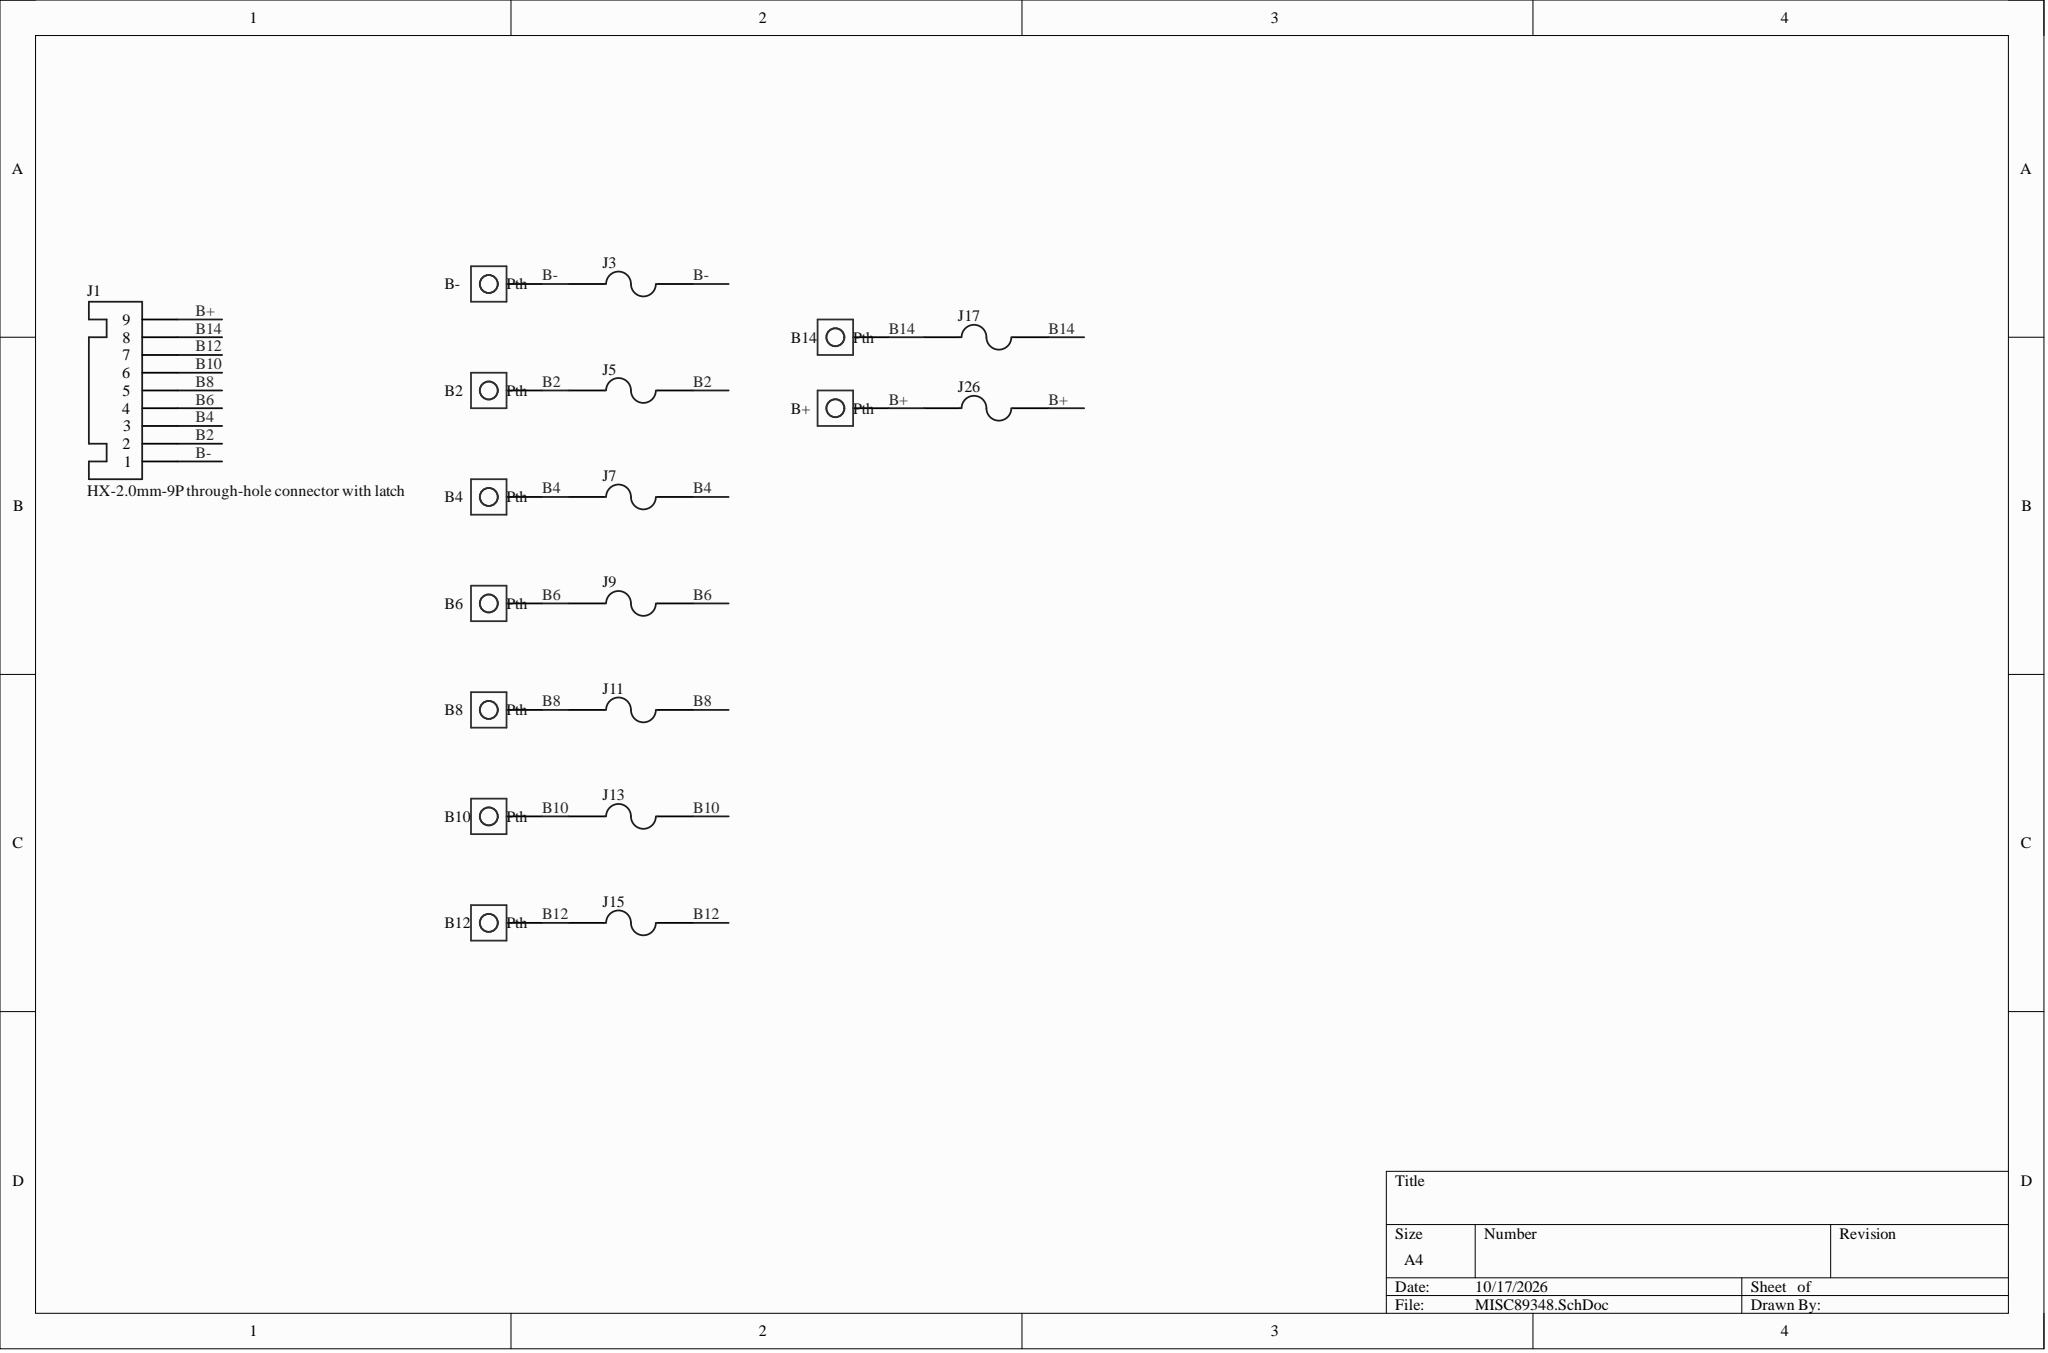Circuit board | Altium Designer | 19 parts | 9 nets
Bill of materials:
Comment,Description,Designator,Footprint,LibRef,Quantity
"Pth","Through-hole pad","B2, B4, B6, B10, B12, B14, B-, B+","55*10*1MM","Pth","8"
"Pth","Through-hole pad","B8","161.5*10*1MM","Pth","1"
"HX-2.0mm-9P through-hole connector with latch","HX-2.54mm-9P through-hole connector with latch","J1","HX2.0-9P","HX-2.54mm-9P直插带扣","1"
"FPC","","J3, J5, J7, J9, J11, J13, J15, J17, J26","异形电阻","FPC","9"
Netlist (Protel format):
[
B2
55*10*1MM
Pth



]
[
B4
55*10*1MM
Pth



]
[
B6
55*10*1MM
Pth



]
[
B8
161.5*10*1MM
Pth



]
[
B10
55*10*1MM
Pth



]
[
B12
55*10*1MM
Pth



]
[
B14
55*10*1MM
Pth



]
[
B+
55*10*1MM
Pth



]
[
B-
55*10*1MM
Pth



]
[
J1
HX2.0-9P
HX-2.0mm-9P through-hole connector with latch



]
[
J3
异形电阻
FPC



]
[
J5
异形电阻
FPC



]
[
J7
异形电阻
FPC



]
[
J9
异形电阻
FPC



]
[
J11
异形电阻
FPC



]
[
J13
异形电阻
FPC



]
[
J15
异形电阻
FPC



]
[
J17
异形电阻
FPC



]
[
J26
异形电阻
FPC



]
(
B-
B--1
J1-1
J3-1
J3-2
)
(
B+
B+-1
J1-9
J26-1
J26-2
)
(
B14
B14-1
J1-8
J17-1
J17-2
)
(
B12
B12-1
J1-7
J15-1
J15-2
)
(
B10
B10-1
J1-6
J13-1
J13-2
)
(
B8
B8-1
J1-5
J11-1
J11-2
)
(
B6
B6-1
J1-4
J9-1
J9-2
)
(
B4
B4-1
J1-3
J7-1
J7-2
)
(
B2
B2-1
J1-2
J5-1
J5-2
)